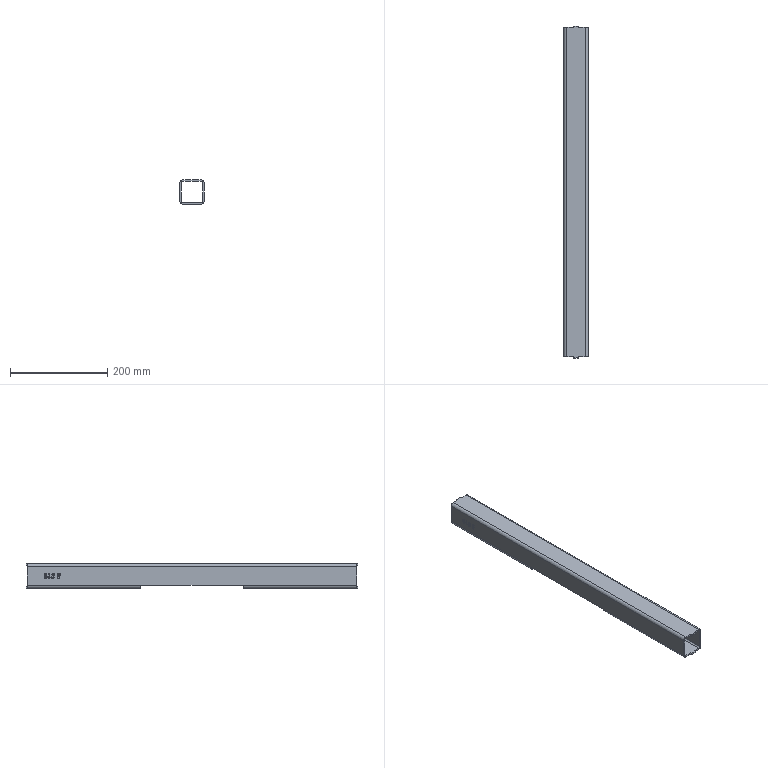Part | SolidWorks | features BaseBody 1 | 1 solid | 91 faces | box 50 x 682 x 50 mm | volume 333028 mm3 | plane 49 | spline 30 | cylinder 12 | commonest cylinder face diameters 6 x6 12 x6